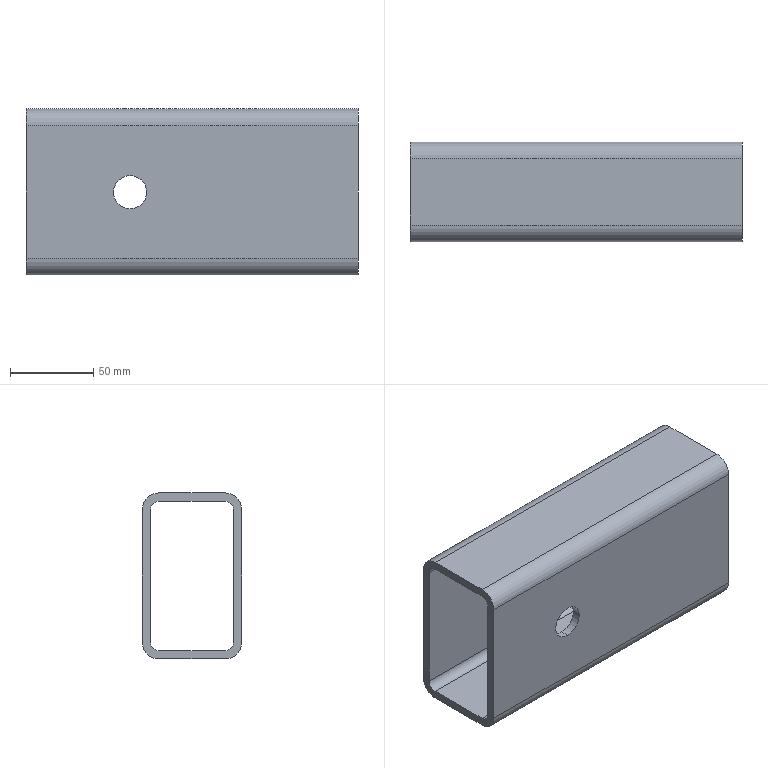Part | SolidWorks | features BaseBody 1 | 1 solid | 22 faces | box 200 x 60 x 100 mm | volume 283982 mm3 | cylinder 12 | plane 10 | commonest cylinder face diameters 20 x8 10 x4
STEP:
#1=CARTESIAN_POINT('',(62.729,5.,9.857));
#2=VERTEX_POINT('',#1);
#3=CARTESIAN_POINT('',(62.729,5.,-10.143));
#4=VERTEX_POINT('',#3);
#5=CARTESIAN_POINT('',(62.729,5.,-0.143));
#6=DIRECTION('',(0.,-1.,0.));
#7=DIRECTION('',(0.,0.,-1.));
#8=AXIS2_PLACEMENT_3D('',#5,#6,#7);
#9=CIRCLE('',#8,10.);
#10=EDGE_CURVE('',#2,#4,#9,.T.);
#11=ORIENTED_EDGE('',*,*,#10,.F.);
#12=CARTESIAN_POINT('',(62.729,0.,9.857));
#13=VERTEX_POINT('',#12);
#14=CARTESIAN_POINT('',(62.729,85.,9.857));
#15=DIRECTION('',(0.,-1.,0.));
#16=VECTOR('',#15,1000.);
#17=LINE('',#14,#16);
#18=EDGE_CURVE('',#2,#13,#17,.T.);
#19=ORIENTED_EDGE('',*,*,#18,.T.);
#20=CARTESIAN_POINT('',(62.729,0.,-10.143));
#21=VERTEX_POINT('',#20);
#22=CARTESIAN_POINT('',(62.729,0.,-0.143));
#23=DIRECTION('',(0.,-1.,0.));
#24=DIRECTION('',(0.,0.,-1.));
#25=AXIS2_PLACEMENT_3D('',#22,#23,#24);
#26=CIRCLE('',#25,10.);
#27=EDGE_CURVE('',#13,#21,#26,.T.);
#28=ORIENTED_EDGE('',*,*,#27,.T.);
#29=CARTESIAN_POINT('',(62.729,85.,-10.143));
#30=DIRECTION('',(0.,-1.,0.));
#31=VECTOR('',#30,1000.);
#32=LINE('',#29,#31);
#33=EDGE_CURVE('',#4,#21,#32,.T.);
#34=ORIENTED_EDGE('',*,*,#33,.F.);
#35=EDGE_LOOP('',(#11,#19,#28,#34));
#36=FACE_OUTER_BOUND('',#35,.T.);
#37=CARTESIAN_POINT('',(62.729,85.,-0.143));
#38=DIRECTION('',(0.,-1.,0.));
#39=DIRECTION('',(0.,0.,-1.));
#40=AXIS2_PLACEMENT_3D('',#37,#38,#39);
#41=CYLINDRICAL_SURFACE('',#40,10.);
#42=ADVANCED_FACE('',(#36),#41,.F.);
#43=CARTESIAN_POINT('',(62.729,60.,-10.143));
#44=VERTEX_POINT('',#43);
#45=CARTESIAN_POINT('',(62.729,60.,9.857));
#46=VERTEX_POINT('',#45);
#47=CARTESIAN_POINT('',(62.729,60.,-0.143));
#48=DIRECTION('',(0.,1.,0.));
#49=DIRECTION('',(0.,0.,-1.));
#50=AXIS2_PLACEMENT_3D('',#47,#48,#49);
#51=CIRCLE('',#50,10.);
#52=EDGE_CURVE('',#44,#46,#51,.T.);
#53=ORIENTED_EDGE('',*,*,#52,.T.);
#54=CARTESIAN_POINT('',(62.729,55.,9.857));
#55=VERTEX_POINT('',#54);
#56=CARTESIAN_POINT('',(62.729,85.,9.857));
#57=DIRECTION('',(0.,-1.,0.));
#58=VECTOR('',#57,1000.);
#59=LINE('',#56,#58);
#60=EDGE_CURVE('',#46,#55,#59,.T.);
#61=ORIENTED_EDGE('',*,*,#60,.T.);
#62=CARTESIAN_POINT('',(62.729,55.,-10.143));
#63=VERTEX_POINT('',#62);
#64=CARTESIAN_POINT('',(62.729,55.,-0.143));
#65=DIRECTION('',(0.,1.,0.));
#66=DIRECTION('',(0.,0.,-1.));
#67=AXIS2_PLACEMENT_3D('',#64,#65,#66);
#68=CIRCLE('',#67,10.);
#69=EDGE_CURVE('',#63,#55,#68,.T.);
#70=ORIENTED_EDGE('',*,*,#69,.F.);
#71=CARTESIAN_POINT('',(62.729,85.,-10.143));
#72=DIRECTION('',(0.,-1.,0.));
#73=VECTOR('',#72,1000.);
#74=LINE('',#71,#73);
#75=EDGE_CURVE('',#44,#63,#74,.T.);
#76=ORIENTED_EDGE('',*,*,#75,.F.);
#77=EDGE_LOOP('',(#53,#61,#70,#76));
#78=FACE_OUTER_BOUND('',#77,.T.);
#79=CARTESIAN_POINT('',(62.729,85.,-0.143));
#80=DIRECTION('',(0.,-1.,0.));
#81=DIRECTION('',(0.,0.,-1.));
#82=AXIS2_PLACEMENT_3D('',#79,#80,#81);
#83=CYLINDRICAL_SURFACE('',#82,10.);
#84=ADVANCED_FACE('',(#78),#83,.F.);
#85=CARTESIAN_POINT('',(200.,0.,-40.));
#86=VERTEX_POINT('',#85);
#87=CARTESIAN_POINT('',(0.,0.,-40.));
#88=VERTEX_POINT('',#87);
#89=CARTESIAN_POINT('',(200.,0.,-40.));
#90=DIRECTION('',(-1.,0.,0.));
#91=VECTOR('',#90,1000.);
#92=LINE('',#89,#91);
#93=EDGE_CURVE('',#86,#88,#92,.T.);
#94=ORIENTED_EDGE('',*,*,#93,.F.);
#95=CARTESIAN_POINT('',(200.,0.,40.));
#96=VERTEX_POINT('',#95);
#97=CARTESIAN_POINT('',(200.,0.,-40.));
#98=DIRECTION('',(0.,0.,-1.));
#99=VECTOR('',#98,1000.);
#100=LINE('',#97,#99);
#101=EDGE_CURVE('',#96,#86,#100,.T.);
#102=ORIENTED_EDGE('',*,*,#101,.F.);
#103=CARTESIAN_POINT('',(0.,0.,40.));
#104=VERTEX_POINT('',#103);
#105=CARTESIAN_POINT('',(200.,0.,40.));
#106=DIRECTION('',(1.,0.,0.));
#107=VECTOR('',#106,1000.);
#108=LINE('',#105,#107);
#109=EDGE_CURVE('',#104,#96,#108,.T.);
#110=ORIENTED_EDGE('',*,*,#109,.F.);
#111=CARTESIAN_POINT('',(0.,0.,-40.));
#112=DIRECTION('',(0.,0.,1.));
#113=VECTOR('',#112,1000.);
#114=LINE('',#111,#113);
#115=EDGE_CURVE('',#88,#104,#114,.T.);
#116=ORIENTED_EDGE('',*,*,#115,.F.);
#117=EDGE_LOOP('',(#94,#102,#110,#116));
#118=FACE_OUTER_BOUND('',#117,.T.);
#119=CARTESIAN_POINT('',(62.729,0.,-0.143));
#120=DIRECTION('',(0.,-1.,0.));
#121=DIRECTION('',(0.,0.,-1.));
#122=AXIS2_PLACEMENT_3D('',#119,#120,#121);
#123=CIRCLE('',#122,10.);
#124=EDGE_CURVE('',#21,#13,#123,.T.);
#125=ORIENTED_EDGE('',*,*,#124,.F.);
#126=ORIENTED_EDGE('',*,*,#27,.F.);
#127=EDGE_LOOP('',(#125,#126));
#128=FACE_BOUND('',#127,.T.);
#129=CARTESIAN_POINT('',(200.,0.,-40.));
#130=DIRECTION('',(0.,1.,0.));
#131=DIRECTION('',(0.,0.,1.));
#132=AXIS2_PLACEMENT_3D('',#129,#130,#131);
#133=PLANE('',#132);
#134=ADVANCED_FACE('',(#118,#128),#133,.F.);
#135=CARTESIAN_POINT('',(0.,60.,-40.));
#136=VERTEX_POINT('',#135);
#137=CARTESIAN_POINT('',(0.,60.,40.));
#138=VERTEX_POINT('',#137);
#139=CARTESIAN_POINT('',(0.,60.,40.));
#140=DIRECTION('',(0.,0.,1.));
#141=VECTOR('',#140,1000.);
#142=LINE('',#139,#141);
#143=EDGE_CURVE('',#136,#138,#142,.T.);
#144=ORIENTED_EDGE('',*,*,#143,.F.);
#145=CARTESIAN_POINT('',(0.,50.,-50.));
#146=VERTEX_POINT('',#145);
#147=CARTESIAN_POINT('',(0.,50.,-40.));
#148=DIRECTION('',(1.,0.,0.));
#149=DIRECTION('',(0.,0.,1.));
#150=AXIS2_PLACEMENT_3D('',#147,#148,#149);
#151=CIRCLE('',#150,10.);
#152=EDGE_CURVE('',#146,#136,#151,.T.);
#153=ORIENTED_EDGE('',*,*,#152,.F.);
#154=CARTESIAN_POINT('',(0.,10.,-50.));
#155=VERTEX_POINT('',#154);
#156=CARTESIAN_POINT('',(0.,50.,-50.));
#157=DIRECTION('',(0.,1.,0.));
#158=VECTOR('',#157,1000.);
#159=LINE('',#156,#158);
#160=EDGE_CURVE('',#155,#146,#159,.T.);
#161=ORIENTED_EDGE('',*,*,#160,.F.);
#162=CARTESIAN_POINT('',(0.,10.,-40.));
#163=DIRECTION('',(1.,0.,0.));
#164=DIRECTION('',(0.,0.,1.));
#165=AXIS2_PLACEMENT_3D('',#162,#163,#164);
#166=CIRCLE('',#165,10.);
#167=EDGE_CURVE('',#88,#155,#166,.T.);
#168=ORIENTED_EDGE('',*,*,#167,.F.);
#169=ORIENTED_EDGE('',*,*,#115,.T.);
#170=CARTESIAN_POINT('',(0.,10.,50.));
#171=VERTEX_POINT('',#170);
#172=CARTESIAN_POINT('',(0.,10.,40.));
#173=DIRECTION('',(1.,0.,0.));
#174=DIRECTION('',(0.,0.,1.));
#175=AXIS2_PLACEMENT_3D('',#172,#173,#174);
#176=CIRCLE('',#175,10.);
#177=EDGE_CURVE('',#171,#104,#176,.T.);
#178=ORIENTED_EDGE('',*,*,#177,.F.);
#179=CARTESIAN_POINT('',(0.,50.,50.));
#180=VERTEX_POINT('',#179);
#181=CARTESIAN_POINT('',(0.,50.,50.));
#182=DIRECTION('',(0.,-1.,0.));
#183=VECTOR('',#182,1000.);
#184=LINE('',#181,#183);
#185=EDGE_CURVE('',#180,#171,#184,.T.);
#186=ORIENTED_EDGE('',*,*,#185,.F.);
#187=CARTESIAN_POINT('',(0.,50.,40.));
#188=DIRECTION('',(1.,0.,0.));
#189=DIRECTION('',(0.,0.,1.));
#190=AXIS2_PLACEMENT_3D('',#187,#188,#189);
#191=CIRCLE('',#190,10.);
#192=EDGE_CURVE('',#138,#180,#191,.T.);
#193=ORIENTED_EDGE('',*,*,#192,.F.);
#194=EDGE_LOOP('',(#144,#153,#161,#168,#169,#178,#186,#193));
#195=FACE_OUTER_BOUND('',#194,.T.);
#196=CARTESIAN_POINT('',(0.,5.,-40.));
#197=VERTEX_POINT('',#196);
#198=CARTESIAN_POINT('',(0.,5.,40.));
#199=VERTEX_POINT('',#198);
#200=CARTESIAN_POINT('',(0.,5.,40.));
#201=DIRECTION('',(0.,0.,1.));
#202=VECTOR('',#201,1000.);
#203=LINE('',#200,#202);
#204=EDGE_CURVE('',#197,#199,#203,.T.);
#205=ORIENTED_EDGE('',*,*,#204,.F.);
#206=CARTESIAN_POINT('',(0.,10.,-45.));
#207=VERTEX_POINT('',#206);
#208=CARTESIAN_POINT('',(0.,10.,-40.));
#209=DIRECTION('',(-1.,0.,0.));
#210=DIRECTION('',(0.,0.,1.));
#211=AXIS2_PLACEMENT_3D('',#208,#209,#210);
#212=CIRCLE('',#211,5.);
#213=EDGE_CURVE('',#207,#197,#212,.T.);
#214=ORIENTED_EDGE('',*,*,#213,.F.);
#215=CARTESIAN_POINT('',(0.,50.,-45.));
#216=VERTEX_POINT('',#215);
#217=CARTESIAN_POINT('',(0.,50.,-45.));
#218=DIRECTION('',(0.,-1.,0.));
#219=VECTOR('',#218,1000.);
#220=LINE('',#217,#219);
#221=EDGE_CURVE('',#216,#207,#220,.T.);
#222=ORIENTED_EDGE('',*,*,#221,.F.);
#223=CARTESIAN_POINT('',(0.,55.,-40.));
#224=VERTEX_POINT('',#223);
#225=CARTESIAN_POINT('',(0.,50.,-40.));
#226=DIRECTION('',(-1.,0.,0.));
#227=DIRECTION('',(0.,0.,1.));
#228=AXIS2_PLACEMENT_3D('',#225,#226,#227);
#229=CIRCLE('',#228,5.);
#230=EDGE_CURVE('',#224,#216,#229,.T.);
#231=ORIENTED_EDGE('',*,*,#230,.F.);
#232=CARTESIAN_POINT('',(0.,55.,40.));
#233=VERTEX_POINT('',#232);
#234=CARTESIAN_POINT('',(0.,55.,40.));
#235=DIRECTION('',(0.,0.,-1.));
#236=VECTOR('',#235,1000.);
#237=LINE('',#234,#236);
#238=EDGE_CURVE('',#233,#224,#237,.T.);
#239=ORIENTED_EDGE('',*,*,#238,.F.);
#240=CARTESIAN_POINT('',(0.,50.,45.));
#241=VERTEX_POINT('',#240);
#242=CARTESIAN_POINT('',(0.,50.,40.));
#243=DIRECTION('',(-1.,0.,0.));
#244=DIRECTION('',(0.,0.,1.));
#245=AXIS2_PLACEMENT_3D('',#242,#243,#244);
#246=CIRCLE('',#245,5.);
#247=EDGE_CURVE('',#241,#233,#246,.T.);
#248=ORIENTED_EDGE('',*,*,#247,.F.);
#249=CARTESIAN_POINT('',(0.,10.,45.));
#250=VERTEX_POINT('',#249);
#251=CARTESIAN_POINT('',(0.,50.,45.));
#252=DIRECTION('',(0.,1.,0.));
#253=VECTOR('',#252,1000.);
#254=LINE('',#251,#253);
#255=EDGE_CURVE('',#250,#241,#254,.T.);
#256=ORIENTED_EDGE('',*,*,#255,.F.);
#257=CARTESIAN_POINT('',(0.,10.,40.));
#258=DIRECTION('',(-1.,0.,0.));
#259=DIRECTION('',(0.,0.,1.));
#260=AXIS2_PLACEMENT_3D('',#257,#258,#259);
#261=CIRCLE('',#260,5.);
#262=EDGE_CURVE('',#199,#250,#261,.T.);
#263=ORIENTED_EDGE('',*,*,#262,.F.);
#264=EDGE_LOOP('',(#205,#214,#222,#231,#239,#248,#256,#263));
#265=FACE_BOUND('',#264,.T.);
#266=CARTESIAN_POINT('',(0.,50.,40.));
#267=DIRECTION('',(1.,0.,0.));
#268=DIRECTION('',(0.,0.,-1.));
#269=AXIS2_PLACEMENT_3D('',#266,#267,#268);
#270=PLANE('',#269);
#271=ADVANCED_FACE('',(#195,#265),#270,.F.);
#272=CARTESIAN_POINT('',(200.,10.,-50.));
#273=VERTEX_POINT('',#272);
#274=CARTESIAN_POINT('',(200.,10.,-40.));
#275=DIRECTION('',(-1.,0.,0.));
#276=DIRECTION('',(0.,0.,1.));
#277=AXIS2_PLACEMENT_3D('',#274,#275,#276);
#278=CIRCLE('',#277,10.);
#279=EDGE_CURVE('',#273,#86,#278,.T.);
#280=ORIENTED_EDGE('',*,*,#279,.T.);
#281=ORIENTED_EDGE('',*,*,#93,.T.);
#282=ORIENTED_EDGE('',*,*,#167,.T.);
#283=CARTESIAN_POINT('',(200.,10.,-50.));
#284=DIRECTION('',(1.,0.,0.));
#285=VECTOR('',#284,1000.);
#286=LINE('',#283,#285);
#287=EDGE_CURVE('',#155,#273,#286,.T.);
#288=ORIENTED_EDGE('',*,*,#287,.T.);
#289=EDGE_LOOP('',(#280,#281,#282,#288));
#290=FACE_OUTER_BOUND('',#289,.T.);
#291=CARTESIAN_POINT('',(200.,10.,-40.));
#292=DIRECTION('',(-1.,0.,0.));
#293=DIRECTION('',(0.,0.,1.));
#294=AXIS2_PLACEMENT_3D('',#291,#292,#293);
#295=CYLINDRICAL_SURFACE('',#294,10.);
#296=ADVANCED_FACE('',(#290),#295,.T.);
#297=CARTESIAN_POINT('',(200.,50.,-50.));
#298=VERTEX_POINT('',#297);
#299=CARTESIAN_POINT('',(200.,60.,-40.));
#300=VERTEX_POINT('',#299);
#301=CARTESIAN_POINT('',(200.,50.,-40.));
#302=DIRECTION('',(1.,0.,0.));
#303=DIRECTION('',(0.,0.,1.));
#304=AXIS2_PLACEMENT_3D('',#301,#302,#303);
#305=CIRCLE('',#304,10.);
#306=EDGE_CURVE('',#298,#300,#305,.T.);
#307=ORIENTED_EDGE('',*,*,#306,.T.);
#308=CARTESIAN_POINT('',(200.,60.,40.));
#309=VERTEX_POINT('',#308);
#310=CARTESIAN_POINT('',(200.,60.,40.));
#311=DIRECTION('',(0.,0.,1.));
#312=VECTOR('',#311,1000.);
#313=LINE('',#310,#312);
#314=EDGE_CURVE('',#300,#309,#313,.T.);
#315=ORIENTED_EDGE('',*,*,#314,.T.);
#316=CARTESIAN_POINT('',(200.,50.,50.));
#317=VERTEX_POINT('',#316);
#318=CARTESIAN_POINT('',(200.,50.,40.));
#319=DIRECTION('',(1.,0.,0.));
#320=DIRECTION('',(0.,0.,1.));
#321=AXIS2_PLACEMENT_3D('',#318,#319,#320);
#322=CIRCLE('',#321,10.);
#323=EDGE_CURVE('',#309,#317,#322,.T.);
#324=ORIENTED_EDGE('',*,*,#323,.T.);
#325=CARTESIAN_POINT('',(200.,10.,50.));
#326=VERTEX_POINT('',#325);
#327=CARTESIAN_POINT('',(200.,50.,50.));
#328=DIRECTION('',(0.,-1.,0.));
#329=VECTOR('',#328,1000.);
#330=LINE('',#327,#329);
#331=EDGE_CURVE('',#317,#326,#330,.T.);
#332=ORIENTED_EDGE('',*,*,#331,.T.);
#333=CARTESIAN_POINT('',(200.,10.,40.));
#334=DIRECTION('',(1.,0.,0.));
#335=DIRECTION('',(0.,0.,1.));
#336=AXIS2_PLACEMENT_3D('',#333,#334,#335);
#337=CIRCLE('',#336,10.);
#338=EDGE_CURVE('',#326,#96,#337,.T.);
#339=ORIENTED_EDGE('',*,*,#338,.T.);
#340=ORIENTED_EDGE('',*,*,#101,.T.);
#341=ORIENTED_EDGE('',*,*,#279,.F.);
#342=CARTESIAN_POINT('',(200.,50.,-50.));
#343=DIRECTION('',(0.,1.,0.));
#344=VECTOR('',#343,1000.);
#345=LINE('',#342,#344);
#346=EDGE_CURVE('',#273,#298,#345,.T.);
#347=ORIENTED_EDGE('',*,*,#346,.T.);
#348=EDGE_LOOP('',(#307,#315,#324,#332,#339,#340,#341,#347));
#349=FACE_OUTER_BOUND('',#348,.T.);
#350=CARTESIAN_POINT('',(200.,10.,-45.));
#351=VERTEX_POINT('',#350);
#352=CARTESIAN_POINT('',(200.,5.,-40.));
#353=VERTEX_POINT('',#352);
#354=CARTESIAN_POINT('',(200.,10.,-40.));
#355=DIRECTION('',(-1.,0.,0.));
#356=DIRECTION('',(0.,0.,1.));
#357=AXIS2_PLACEMENT_3D('',#354,#355,#356);
#358=CIRCLE('',#357,5.);
#359=EDGE_CURVE('',#351,#353,#358,.T.);
#360=ORIENTED_EDGE('',*,*,#359,.T.);
#361=CARTESIAN_POINT('',(200.,5.,40.));
#362=VERTEX_POINT('',#361);
#363=CARTESIAN_POINT('',(200.,5.,40.));
#364=DIRECTION('',(0.,0.,1.));
#365=VECTOR('',#364,1000.);
#366=LINE('',#363,#365);
#367=EDGE_CURVE('',#353,#362,#366,.T.);
#368=ORIENTED_EDGE('',*,*,#367,.T.);
#369=CARTESIAN_POINT('',(200.,10.,45.));
#370=VERTEX_POINT('',#369);
#371=CARTESIAN_POINT('',(200.,10.,40.));
#372=DIRECTION('',(-1.,0.,0.));
#373=DIRECTION('',(0.,0.,1.));
#374=AXIS2_PLACEMENT_3D('',#371,#372,#373);
#375=CIRCLE('',#374,5.);
#376=EDGE_CURVE('',#362,#370,#375,.T.);
#377=ORIENTED_EDGE('',*,*,#376,.T.);
#378=CARTESIAN_POINT('',(200.,50.,45.));
#379=VERTEX_POINT('',#378);
#380=CARTESIAN_POINT('',(200.,50.,45.));
#381=DIRECTION('',(0.,1.,0.));
#382=VECTOR('',#381,1000.);
#383=LINE('',#380,#382);
#384=EDGE_CURVE('',#370,#379,#383,.T.);
#385=ORIENTED_EDGE('',*,*,#384,.T.);
#386=CARTESIAN_POINT('',(200.,55.,40.));
#387=VERTEX_POINT('',#386);
#388=CARTESIAN_POINT('',(200.,50.,40.));
#389=DIRECTION('',(-1.,0.,0.));
#390=DIRECTION('',(0.,0.,1.));
#391=AXIS2_PLACEMENT_3D('',#388,#389,#390);
#392=CIRCLE('',#391,5.);
#393=EDGE_CURVE('',#379,#387,#392,.T.);
#394=ORIENTED_EDGE('',*,*,#393,.T.);
#395=CARTESIAN_POINT('',(200.,55.,-40.));
#396=VERTEX_POINT('',#395);
#397=CARTESIAN_POINT('',(200.,55.,40.));
#398=DIRECTION('',(0.,0.,-1.));
#399=VECTOR('',#398,1000.);
#400=LINE('',#397,#399);
#401=EDGE_CURVE('',#387,#396,#400,.T.);
#402=ORIENTED_EDGE('',*,*,#401,.T.);
#403=CARTESIAN_POINT('',(200.,50.,-45.));
#404=VERTEX_POINT('',#403);
#405=CARTESIAN_POINT('',(200.,50.,-40.));
#406=DIRECTION('',(-1.,0.,0.));
#407=DIRECTION('',(0.,0.,1.));
#408=AXIS2_PLACEMENT_3D('',#405,#406,#407);
#409=CIRCLE('',#408,5.);
#410=EDGE_CURVE('',#396,#404,#409,.T.);
#411=ORIENTED_EDGE('',*,*,#410,.T.);
#412=CARTESIAN_POINT('',(200.,50.,-45.));
#413=DIRECTION('',(0.,-1.,0.));
#414=VECTOR('',#413,1000.);
#415=LINE('',#412,#414);
#416=EDGE_CURVE('',#404,#351,#415,.T.);
#417=ORIENTED_EDGE('',*,*,#416,.T.);
#418=EDGE_LOOP('',(#360,#368,#377,#385,#394,#402,#411,#417));
#419=FACE_BOUND('',#418,.T.);
#420=CARTESIAN_POINT('',(200.,50.,40.));
#421=DIRECTION('',(1.,0.,0.));
#422=DIRECTION('',(0.,0.,-1.));
#423=AXIS2_PLACEMENT_3D('',#420,#421,#422);
#424=PLANE('',#423);
#425=ADVANCED_FACE('',(#349,#419),#424,.T.);
#426=ORIENTED_EDGE('',*,*,#338,.F.);
#427=CARTESIAN_POINT('',(200.,10.,50.));
#428=DIRECTION('',(-1.,0.,0.));
#429=VECTOR('',#428,1000.);
#430=LINE('',#427,#429);
#431=EDGE_CURVE('',#326,#171,#430,.T.);
#432=ORIENTED_EDGE('',*,*,#431,.T.);
#433=ORIENTED_EDGE('',*,*,#177,.T.);
#434=ORIENTED_EDGE('',*,*,#109,.T.);
#435=EDGE_LOOP('',(#426,#432,#433,#434));
#436=FACE_OUTER_BOUND('',#435,.T.);
#437=CARTESIAN_POINT('',(200.,10.,40.));
#438=DIRECTION('',(-1.,0.,0.));
#439=DIRECTION('',(0.,0.,1.));
#440=AXIS2_PLACEMENT_3D('',#437,#438,#439);
#441=CYLINDRICAL_SURFACE('',#440,10.);
#442=ADVANCED_FACE('',(#436),#441,.T.);
#443=ORIENTED_EDGE('',*,*,#18,.F.);
#444=CARTESIAN_POINT('',(62.729,5.,-0.143));
#445=DIRECTION('',(0.,-1.,0.));
#446=DIRECTION('',(0.,0.,-1.));
#447=AXIS2_PLACEMENT_3D('',#444,#445,#446);
#448=CIRCLE('',#447,10.);
#449=EDGE_CURVE('',#4,#2,#448,.T.);
#450=ORIENTED_EDGE('',*,*,#449,.F.);
#451=ORIENTED_EDGE('',*,*,#33,.T.);
#452=ORIENTED_EDGE('',*,*,#124,.T.);
#453=EDGE_LOOP('',(#443,#450,#451,#452));
#454=FACE_OUTER_BOUND('',#453,.T.);
#455=CARTESIAN_POINT('',(62.729,85.,-0.143));
#456=DIRECTION('',(0.,-1.,0.));
#457=DIRECTION('',(0.,0.,-1.));
#458=AXIS2_PLACEMENT_3D('',#455,#456,#457);
#459=CYLINDRICAL_SURFACE('',#458,10.);
#460=ADVANCED_FACE('',(#454),#459,.F.);
#461=ORIENTED_EDGE('',*,*,#323,.F.);
#462=CARTESIAN_POINT('',(200.,60.,40.));
#463=DIRECTION('',(-1.,0.,0.));
#464=VECTOR('',#463,1000.);
#465=LINE('',#462,#464);
#466=EDGE_CURVE('',#309,#138,#465,.T.);
#467=ORIENTED_EDGE('',*,*,#466,.T.);
#468=ORIENTED_EDGE('',*,*,#192,.T.);
#469=CARTESIAN_POINT('',(200.,50.,50.));
#470=DIRECTION('',(1.,0.,0.));
#471=VECTOR('',#470,1000.);
#472=LINE('',#469,#471);
#473=EDGE_CURVE('',#180,#317,#472,.T.);
#474=ORIENTED_EDGE('',*,*,#473,.T.);
#475=EDGE_LOOP('',(#461,#467,#468,#474));
#476=FACE_OUTER_BOUND('',#475,.T.);
#477=CARTESIAN_POINT('',(200.,50.,40.));
#478=DIRECTION('',(-1.,0.,0.));
#479=DIRECTION('',(0.,0.,1.));
#480=AXIS2_PLACEMENT_3D('',#477,#478,#479);
#481=CYLINDRICAL_SURFACE('',#480,10.);
#482=ADVANCED_FACE('',(#476),#481,.T.);
#483=ORIENTED_EDGE('',*,*,#466,.F.);
#484=ORIENTED_EDGE('',*,*,#314,.F.);
#485=CARTESIAN_POINT('',(200.,60.,-40.));
#486=DIRECTION('',(1.,0.,0.));
#487=VECTOR('',#486,1000.);
#488=LINE('',#485,#487);
#489=EDGE_CURVE('',#136,#300,#488,.T.);
#490=ORIENTED_EDGE('',*,*,#489,.F.);
#491=ORIENTED_EDGE('',*,*,#143,.T.);
#492=EDGE_LOOP('',(#483,#484,#490,#491));
#493=FACE_OUTER_BOUND('',#492,.T.);
#494=ORIENTED_EDGE('',*,*,#52,.F.);
#495=CARTESIAN_POINT('',(62.729,60.,-0.143));
#496=DIRECTION('',(0.,1.,0.));
#497=DIRECTION('',(0.,0.,-1.));
#498=AXIS2_PLACEMENT_3D('',#495,#496,#497);
#499=CIRCLE('',#498,10.);
#500=EDGE_CURVE('',#46,#44,#499,.T.);
#501=ORIENTED_EDGE('',*,*,#500,.F.);
#502=EDGE_LOOP('',(#494,#501));
#503=FACE_BOUND('',#502,.T.);
#504=CARTESIAN_POINT('',(200.,60.,40.));
#505=DIRECTION('',(0.,-1.,0.));
#506=DIRECTION('',(0.,0.,-1.));
#507=AXIS2_PLACEMENT_3D('',#504,#505,#506);
#508=PLANE('',#507);
#509=ADVANCED_FACE('',(#493,#503),#508,.F.);
#510=ORIENTED_EDGE('',*,*,#306,.F.);
#511=CARTESIAN_POINT('',(200.,50.,-50.));
#512=DIRECTION('',(-1.,0.,0.));
#513=VECTOR('',#512,1000.);
#514=LINE('',#511,#513);
#515=EDGE_CURVE('',#298,#146,#514,.T.);
#516=ORIENTED_EDGE('',*,*,#515,.T.);
#517=ORIENTED_EDGE('',*,*,#152,.T.);
#518=ORIENTED_EDGE('',*,*,#489,.T.);
#519=EDGE_LOOP('',(#510,#516,#517,#518));
#520=FACE_OUTER_BOUND('',#519,.T.);
#521=CARTESIAN_POINT('',(200.,50.,-40.));
#522=DIRECTION('',(-1.,0.,0.));
#523=DIRECTION('',(0.,0.,1.));
#524=AXIS2_PLACEMENT_3D('',#521,#522,#523);
#525=CYLINDRICAL_SURFACE('',#524,10.);
#526=ADVANCED_FACE('',(#520),#525,.T.);
#527=ORIENTED_EDGE('',*,*,#515,.F.);
#528=ORIENTED_EDGE('',*,*,#346,.F.);
#529=ORIENTED_EDGE('',*,*,#287,.F.);
#530=ORIENTED_EDGE('',*,*,#160,.T.);
#531=EDGE_LOOP('',(#527,#528,#529,#530));
#532=FACE_OUTER_BOUND('',#531,.T.);
#533=CARTESIAN_POINT('',(200.,10.,-50.));
#534=DIRECTION('',(0.,0.,1.));
#535=DIRECTION('',(0.,-1.,0.));
#536=AXIS2_PLACEMENT_3D('',#533,#534,#535);
#537=PLANE('',#536);
#538=ADVANCED_FACE('',(#532),#537,.F.);
#539=ORIENTED_EDGE('',*,*,#431,.F.);
#540=ORIENTED_EDGE('',*,*,#331,.F.);
#541=ORIENTED_EDGE('',*,*,#473,.F.);
#542=ORIENTED_EDGE('',*,*,#185,.T.);
#543=EDGE_LOOP('',(#539,#540,#541,#542));
#544=FACE_OUTER_BOUND('',#543,.T.);
#545=CARTESIAN_POINT('',(200.,50.,50.));
#546=DIRECTION('',(0.,0.,-1.));
#547=DIRECTION('',(0.,1.,0.));
#548=AXIS2_PLACEMENT_3D('',#545,#546,#547);
#549=PLANE('',#548);
#550=ADVANCED_FACE('',(#544),#549,.F.);
#551=CARTESIAN_POINT('',(200.,10.,45.));
#552=DIRECTION('',(-1.,0.,0.));
#553=VECTOR('',#552,1000.);
#554=LINE('',#551,#553);
#555=EDGE_CURVE('',#370,#250,#554,.T.);
#556=ORIENTED_EDGE('',*,*,#555,.F.);
#557=ORIENTED_EDGE('',*,*,#376,.F.);
#558=CARTESIAN_POINT('',(200.,5.,40.));
#559=DIRECTION('',(1.,0.,0.));
#560=VECTOR('',#559,1000.);
#561=LINE('',#558,#560);
#562=EDGE_CURVE('',#199,#362,#561,.T.);
#563=ORIENTED_EDGE('',*,*,#562,.F.);
#564=ORIENTED_EDGE('',*,*,#262,.T.);
#565=EDGE_LOOP('',(#556,#557,#563,#564));
#566=FACE_OUTER_BOUND('',#565,.T.);
#567=CARTESIAN_POINT('',(200.,10.,40.));
#568=DIRECTION('',(-1.,0.,0.));
#569=DIRECTION('',(0.,0.,1.));
#570=AXIS2_PLACEMENT_3D('',#567,#568,#569);
#571=CYLINDRICAL_SURFACE('',#570,5.);
#572=ADVANCED_FACE('',(#566),#571,.F.);
#573=ORIENTED_EDGE('',*,*,#367,.F.);
#574=CARTESIAN_POINT('',(200.,5.,-40.));
#575=DIRECTION('',(-1.,0.,0.));
#576=VECTOR('',#575,1000.);
#577=LINE('',#574,#576);
#578=EDGE_CURVE('',#353,#197,#577,.T.);
#579=ORIENTED_EDGE('',*,*,#578,.T.);
#580=ORIENTED_EDGE('',*,*,#204,.T.);
#581=ORIENTED_EDGE('',*,*,#562,.T.);
#582=EDGE_LOOP('',(#573,#579,#580,#581));
#583=FACE_OUTER_BOUND('',#582,.T.);
#584=ORIENTED_EDGE('',*,*,#449,.T.);
#585=ORIENTED_EDGE('',*,*,#10,.T.);
#586=EDGE_LOOP('',(#584,#585));
#587=FACE_BOUND('',#586,.T.);
#588=CARTESIAN_POINT('',(200.,5.,-40.));
#589=DIRECTION('',(0.,1.,0.));
#590=DIRECTION('',(0.,0.,1.));
#591=AXIS2_PLACEMENT_3D('',#588,#589,#590);
#592=PLANE('',#591);
#593=ADVANCED_FACE('',(#583,#587),#592,.T.);
#594=ORIENTED_EDGE('',*,*,#578,.F.);
#595=ORIENTED_EDGE('',*,*,#359,.F.);
#596=CARTESIAN_POINT('',(200.,10.,-45.));
#597=DIRECTION('',(1.,0.,0.));
#598=VECTOR('',#597,1000.);
#599=LINE('',#596,#598);
#600=EDGE_CURVE('',#207,#351,#599,.T.);
#601=ORIENTED_EDGE('',*,*,#600,.F.);
#602=ORIENTED_EDGE('',*,*,#213,.T.);
#603=EDGE_LOOP('',(#594,#595,#601,#602));
#604=FACE_OUTER_BOUND('',#603,.T.);
#605=CARTESIAN_POINT('',(200.,10.,-40.));
#606=DIRECTION('',(-1.,0.,0.));
#607=DIRECTION('',(0.,0.,1.));
#608=AXIS2_PLACEMENT_3D('',#605,#606,#607);
#609=CYLINDRICAL_SURFACE('',#608,5.);
#610=ADVANCED_FACE('',(#604),#609,.F.);
#611=ORIENTED_EDGE('',*,*,#416,.F.);
#612=CARTESIAN_POINT('',(200.,50.,-45.));
#613=DIRECTION('',(-1.,0.,0.));
#614=VECTOR('',#613,1000.);
#615=LINE('',#612,#614);
#616=EDGE_CURVE('',#404,#216,#615,.T.);
#617=ORIENTED_EDGE('',*,*,#616,.T.);
#618=ORIENTED_EDGE('',*,*,#221,.T.);
#619=ORIENTED_EDGE('',*,*,#600,.T.);
#620=EDGE_LOOP('',(#611,#617,#618,#619));
#621=FACE_OUTER_BOUND('',#620,.T.);
#622=CARTESIAN_POINT('',(200.,10.,-45.));
#623=DIRECTION('',(0.,0.,1.));
#624=DIRECTION('',(0.,-1.,0.));
#625=AXIS2_PLACEMENT_3D('',#622,#623,#624);
#626=PLANE('',#625);
#627=ADVANCED_FACE('',(#621),#626,.T.);
#628=ORIENTED_EDGE('',*,*,#616,.F.);
#629=ORIENTED_EDGE('',*,*,#410,.F.);
#630=CARTESIAN_POINT('',(200.,55.,-40.));
#631=DIRECTION('',(1.,0.,0.));
#632=VECTOR('',#631,1000.);
#633=LINE('',#630,#632);
#634=EDGE_CURVE('',#224,#396,#633,.T.);
#635=ORIENTED_EDGE('',*,*,#634,.F.);
#636=ORIENTED_EDGE('',*,*,#230,.T.);
#637=EDGE_LOOP('',(#628,#629,#635,#636));
#638=FACE_OUTER_BOUND('',#637,.T.);
#639=CARTESIAN_POINT('',(200.,50.,-40.));
#640=DIRECTION('',(-1.,0.,0.));
#641=DIRECTION('',(0.,0.,1.));
#642=AXIS2_PLACEMENT_3D('',#639,#640,#641);
#643=CYLINDRICAL_SURFACE('',#642,5.);
#644=ADVANCED_FACE('',(#638),#643,.F.);
#645=ORIENTED_EDGE('',*,*,#401,.F.);
#646=CARTESIAN_POINT('',(200.,55.,40.));
#647=DIRECTION('',(-1.,0.,0.));
#648=VECTOR('',#647,1000.);
#649=LINE('',#646,#648);
#650=EDGE_CURVE('',#387,#233,#649,.T.);
#651=ORIENTED_EDGE('',*,*,#650,.T.);
#652=ORIENTED_EDGE('',*,*,#238,.T.);
#653=ORIENTED_EDGE('',*,*,#634,.T.);
#654=EDGE_LOOP('',(#645,#651,#652,#653));
#655=FACE_OUTER_BOUND('',#654,.T.);
#656=ORIENTED_EDGE('',*,*,#69,.T.);
#657=CARTESIAN_POINT('',(62.729,55.,-0.143));
#658=DIRECTION('',(0.,1.,0.));
#659=DIRECTION('',(0.,0.,-1.));
#660=AXIS2_PLACEMENT_3D('',#657,#658,#659);
#661=CIRCLE('',#660,10.);
#662=EDGE_CURVE('',#55,#63,#661,.T.);
#663=ORIENTED_EDGE('',*,*,#662,.T.);
#664=EDGE_LOOP('',(#656,#663));
#665=FACE_BOUND('',#664,.T.);
#666=CARTESIAN_POINT('',(200.,55.,40.));
#667=DIRECTION('',(0.,-1.,0.));
#668=DIRECTION('',(0.,0.,-1.));
#669=AXIS2_PLACEMENT_3D('',#666,#667,#668);
#670=PLANE('',#669);
#671=ADVANCED_FACE('',(#655,#665),#670,.T.);
#672=ORIENTED_EDGE('',*,*,#650,.F.);
#673=ORIENTED_EDGE('',*,*,#393,.F.);
#674=CARTESIAN_POINT('',(200.,50.,45.));
#675=DIRECTION('',(1.,0.,0.));
#676=VECTOR('',#675,1000.);
#677=LINE('',#674,#676);
#678=EDGE_CURVE('',#241,#379,#677,.T.);
#679=ORIENTED_EDGE('',*,*,#678,.F.);
#680=ORIENTED_EDGE('',*,*,#247,.T.);
#681=EDGE_LOOP('',(#672,#673,#679,#680));
#682=FACE_OUTER_BOUND('',#681,.T.);
#683=CARTESIAN_POINT('',(200.,50.,40.));
#684=DIRECTION('',(-1.,0.,0.));
#685=DIRECTION('',(0.,0.,1.));
#686=AXIS2_PLACEMENT_3D('',#683,#684,#685);
#687=CYLINDRICAL_SURFACE('',#686,5.);
#688=ADVANCED_FACE('',(#682),#687,.F.);
#689=ORIENTED_EDGE('',*,*,#384,.F.);
#690=ORIENTED_EDGE('',*,*,#555,.T.);
#691=ORIENTED_EDGE('',*,*,#255,.T.);
#692=ORIENTED_EDGE('',*,*,#678,.T.);
#693=EDGE_LOOP('',(#689,#690,#691,#692));
#694=FACE_OUTER_BOUND('',#693,.T.);
#695=CARTESIAN_POINT('',(200.,50.,45.));
#696=DIRECTION('',(0.,0.,-1.));
#697=DIRECTION('',(0.,1.,0.));
#698=AXIS2_PLACEMENT_3D('',#695,#696,#697);
#699=PLANE('',#698);
#700=ADVANCED_FACE('',(#694),#699,.T.);
#701=ORIENTED_EDGE('',*,*,#60,.F.);
#702=ORIENTED_EDGE('',*,*,#500,.T.);
#703=ORIENTED_EDGE('',*,*,#75,.T.);
#704=ORIENTED_EDGE('',*,*,#662,.F.);
#705=EDGE_LOOP('',(#701,#702,#703,#704));
#706=FACE_OUTER_BOUND('',#705,.T.);
#707=CARTESIAN_POINT('',(62.729,85.,-0.143));
#708=DIRECTION('',(0.,-1.,0.));
#709=DIRECTION('',(0.,0.,-1.));
#710=AXIS2_PLACEMENT_3D('',#707,#708,#709);
#711=CYLINDRICAL_SURFACE('',#710,10.);
#712=ADVANCED_FACE('',(#706),#711,.F.);
#713=CLOSED_SHELL('',(#42,#84,#134,#271,#296,#425,#442,#460,#482,#509,#526,#538,#550,#572,#593,#610,#627,#644,#671,#688,#700,#712));
#714=MANIFOLD_SOLID_BREP('',#713);
#715=CARTESIAN_POINT('',(0.,0.,0.));
#716=DIRECTION('',(0.,0.,1.));
#717=DIRECTION('',(1.,0.,0.));
#718=AXIS2_PLACEMENT_3D('',#715,#716,#717);
#719=(LENGTH_UNIT()NAMED_UNIT(*)SI_UNIT(.MILLI.,.METRE.));
#720=UNCERTAINTY_MEASURE_WITH_UNIT(LENGTH_MEASURE(0.00001),#719,'','');
#721=(NAMED_UNIT(*)PLANE_ANGLE_UNIT()SI_UNIT($,.RADIAN.));
#722=(NAMED_UNIT(*)SI_UNIT($,.STERADIAN.)SOLID_ANGLE_UNIT());
#723=(GEOMETRIC_REPRESENTATION_CONTEXT(3)GLOBAL_UNCERTAINTY_ASSIGNED_CONTEXT((#720))GLOBAL_UNIT_ASSIGNED_CONTEXT((#719,#721,#722))REPRESENTATION_CONTEXT('',''));
#724=ADVANCED_BREP_SHAPE_REPRESENTATION('',(#714,#718),#723);